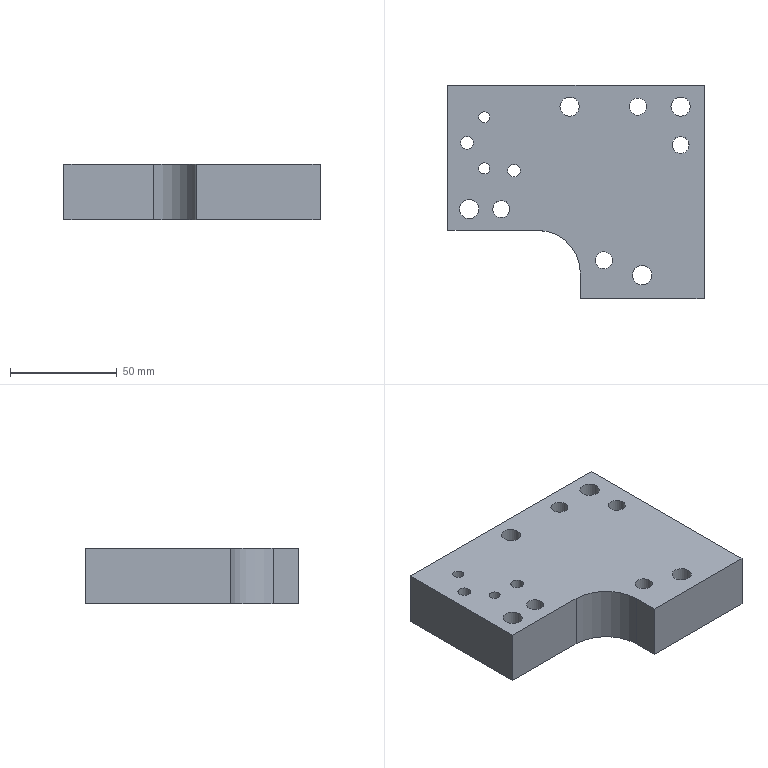Part | STEP file | 102_id46_x_t | 1 solid | 46 faces | box 120 x 100 x 26 mm | volume 237897 mm3 | cylinder 22 | plane 14 | cone 10 | commonest cylinder face diameters 8 x4 9 x4 14 x4 8.5 x3 6 x2 6.8 x2